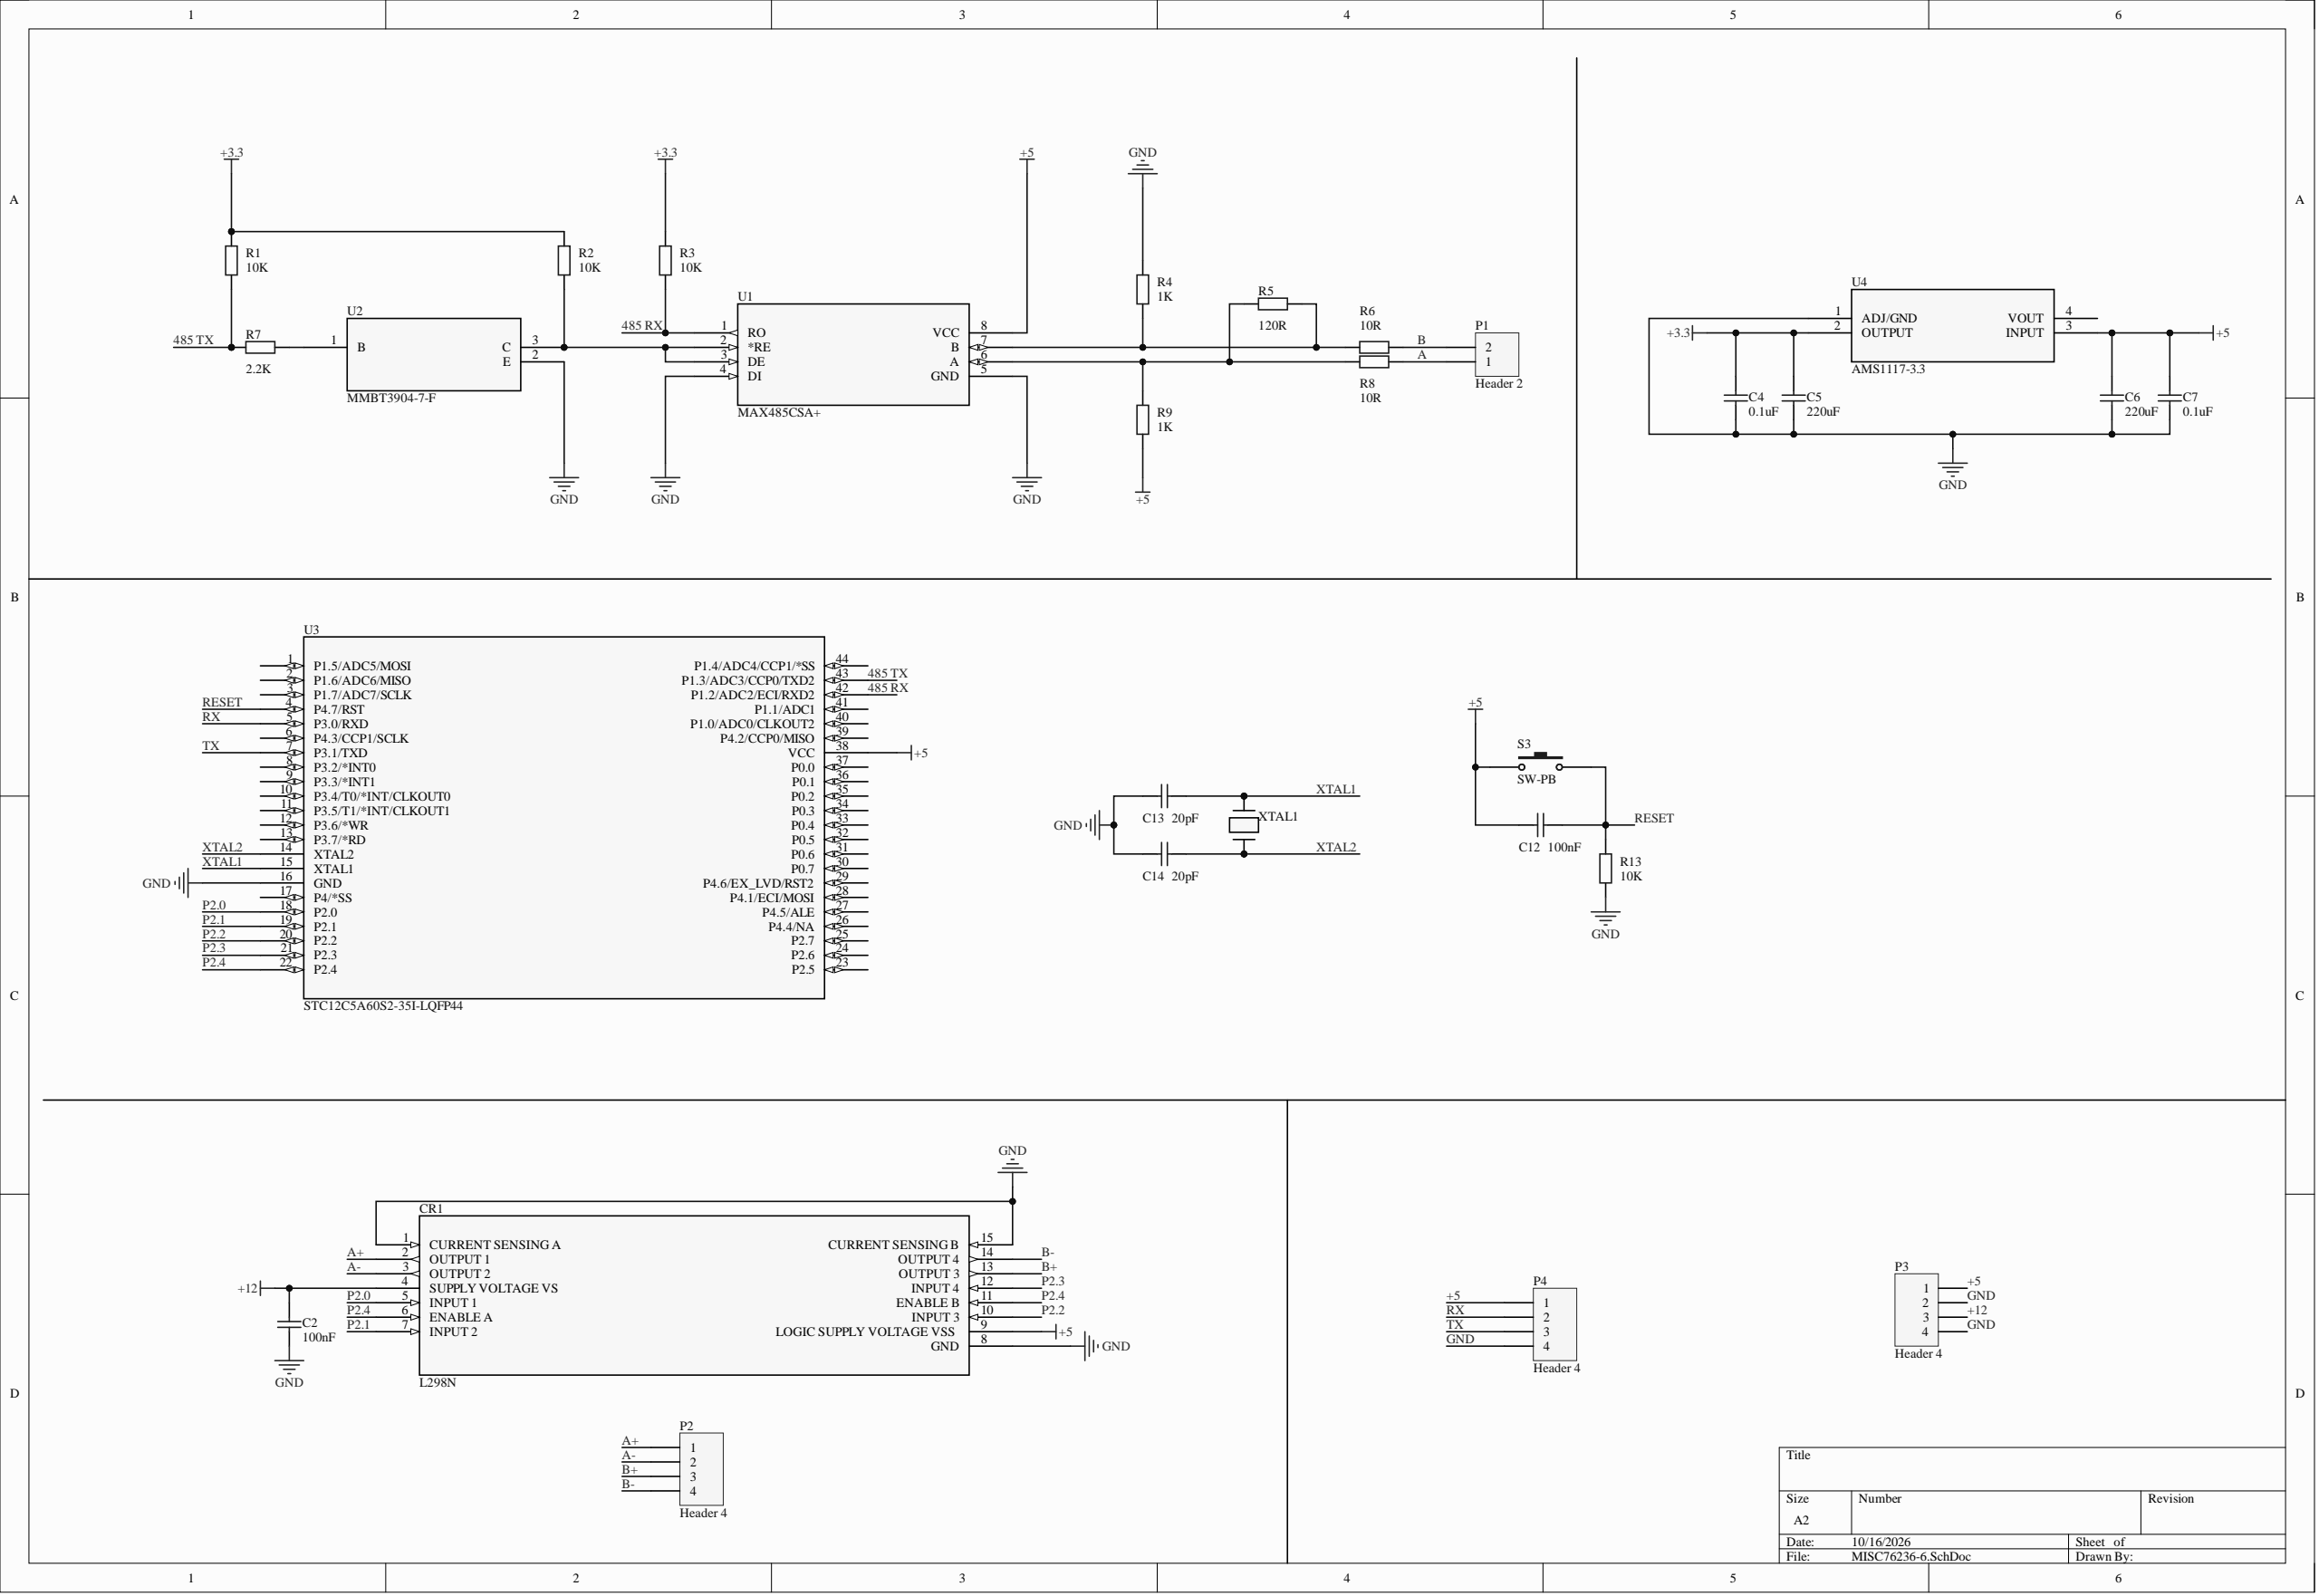Circuit board | Altium Designer | 29 parts | 26 nets
Bill of materials:
Comment,Description,Designator,Footprint,LibRef,Quantity
"Cap","Capacitor","C2, C4, C5, C6, C7, C12, C13, C14","RAD-0.3","Cap","8"
"L298N","No Description Available","CR1","Multiwatt15_V_STM","L298N","1"
"Header 2","Header, 2-Pin","P1","HDR1X2","Header 2","1"
"Header 4","Header, 4-Pin","P2, P3, P4","HDR1X4","Header 4","3"
"Res2","Resistor","R1, R2, R3, R4, R5, R6, R7, R8, R9, R13","AXIAL-0.4","Res2","10"
"SW-PB","Switch","S3","SPST-2","SW-PB","1"
"MAX485CSA+","No Description Available","U1","21-0041B_8_MXM","MAX485CSA+","1"
"MMBT3904-7-F","No Description Available","U2","SOT-23_1_DIO","MMBT3904-7-F","1"
"STC12C5A60S2-35I-LQFP44","No Description Available","U3","LQFP44_STC89_STC_SCM","STC12C5A60S2-35I-LQFP44","1"
"AMS1117-3.3","No Description Available","U4","TS3B_TEX","AMS1117-3.3","1"
"HC49S-11.059-30-50-70-30-ATF","No Description Available","XTAL1","XTAL_HC49S_MTC","HC49S-11.059-30-50-70-30-ATF","1"
Netlist (Protel format):
[
C2
RAD-0.3
Cap



]
[
C4
RAD-0.3
Cap



]
[
C5
RAD-0.3
Cap



]
[
C6
RAD-0.3
Cap



]
[
C7
RAD-0.3
Cap



]
[
C12
RAD-0.3
Cap



]
[
C13
RAD-0.3
Cap



]
[
C14
RAD-0.3
Cap



]
[
CR1
Multiwatt15_V_STM
L298N



]
[
P1
HDR1X2
Header 2



]
[
P2
HDR1X4
Header 4



]
[
P3
HDR1X4
Header 4



]
[
P4
HDR1X4
Header 4



]
[
R1
AXIAL-0.4
Res2



]
[
R2
AXIAL-0.4
Res2



]
[
R3
AXIAL-0.4
Res2



]
[
R4
AXIAL-0.4
Res2



]
[
R5
AXIAL-0.4
Res2



]
[
R6
AXIAL-0.4
Res2



]
[
R7
AXIAL-0.4
Res2



]
[
R8
AXIAL-0.4
Res2



]
[
R9
AXIAL-0.4
Res2



]
[
R13
AXIAL-0.4
Res2



]
[
S3
SPST-2
SW-PB



]
[
U1
21-0041B_8_MXM
MAX485CSA+



]
[
U2
SOT-23_1_DIO
MMBT3904-7-F



]
[
U3
LQFP44_STC89_STC_SCM
STC12C5A60S2-35I-LQFP44



]
[
U4
TS3B_TEX
AMS1117-3.3



]
[
XTAL1
XTAL_HC49S_MTC
HC49S-11.0592-30-50-70-30-ATF



]
(
XTAL2
C14-2
U3-14
XTAL1-1
)
(
XTAL1
C13-2
U3-15
XTAL1-2
)
(
TX
P4-3
U3-7
)
(
RX
P4-2
U3-5
)
(
RESET
C12-2
R13-2
S3-2
U3-4
)
(
P2.4
CR1-6
CR1-11
U3-22
)
(
P2.3
CR1-12
U3-21
)
(
P2.2
CR1-10
U3-20
)
(
P2.1
CR1-7
U3-19
)
(
P2.0
CR1-5
U3-18
)
(
NetR7_2
R7-2
U2-1
)
(
NetR5_1
R5-1
R8-1
R9-2
U1-6
)
(
NetR4_1
R4-1
R5-2
R6-1
U1-7
)
(
NetR2_1
R2-1
U1-2
U1-3
U2-3
)
(
GND
C2-1
C4-1
C5-1
C6-1
C7-1
C13-1
C14-1
CR1-1
CR1-8
CR1-15
P3-2
P3-4
P4-4
R4-2
R13-1
U1-4
U1-5
U2-2
U3-16
U4-1
)
(
B-
CR1-14
P2-4
)
(
B+
CR1-13
P2-3
)
(
B
P1-2
R6-2
)
(
A-
CR1-3
P2-2
)
(
A+
CR1-2
P2-1
)
(
A
P1-1
R8-2
)
(
+12
C2-2
CR1-4
P3-3
)
(
+5
C6-2
C7-2
C12-1
CR1-9
P3-1
P4-1
R9-1
S3-1
U1-8
U3-38
U4-3
)
(
+3.3
C4-2
C5-2
R1-2
R2-2
R3-2
U4-2
)
(
485 TX
R1-1
R7-1
U3-43
)
(
485 RX
R3-1
U1-1
U3-42
)